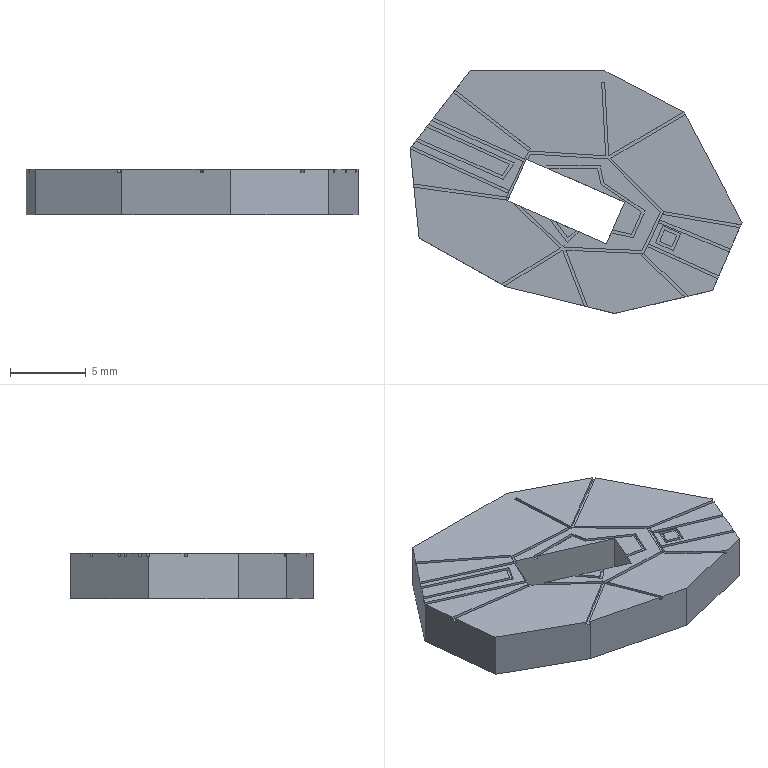Part | SolidWorks | features BaseBody 1 | 1 solid | 117 faces | box 21.888 x 16.021 x 3 mm | volume 729.931 mm3 | plane 110 | spline 7